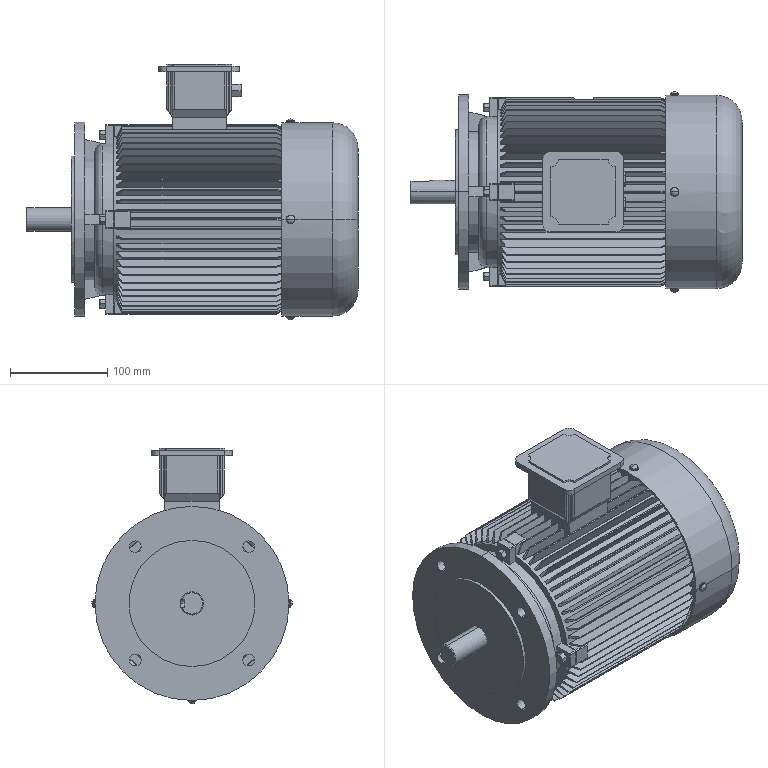Part | SolidWorks | features Boss 15, Cut 5, Revolution 5, Fillet 4, Chamfer 3, CirPattern 3, RevCut 2, 3DProfileFeature 1, MirrorPattern 1, MoveCopyBody 1 | 2 solids | 662 faces | box 342 x 207 x 263.5 mm | volume 6736736 mm3 | plane 395 | cone 154 | cylinder 91 | torus 14 | sphere 8 | commonest cylinder face diameters 3.937 x10 171 x10 7 x9 8.2 x8 9 x8 12 x8